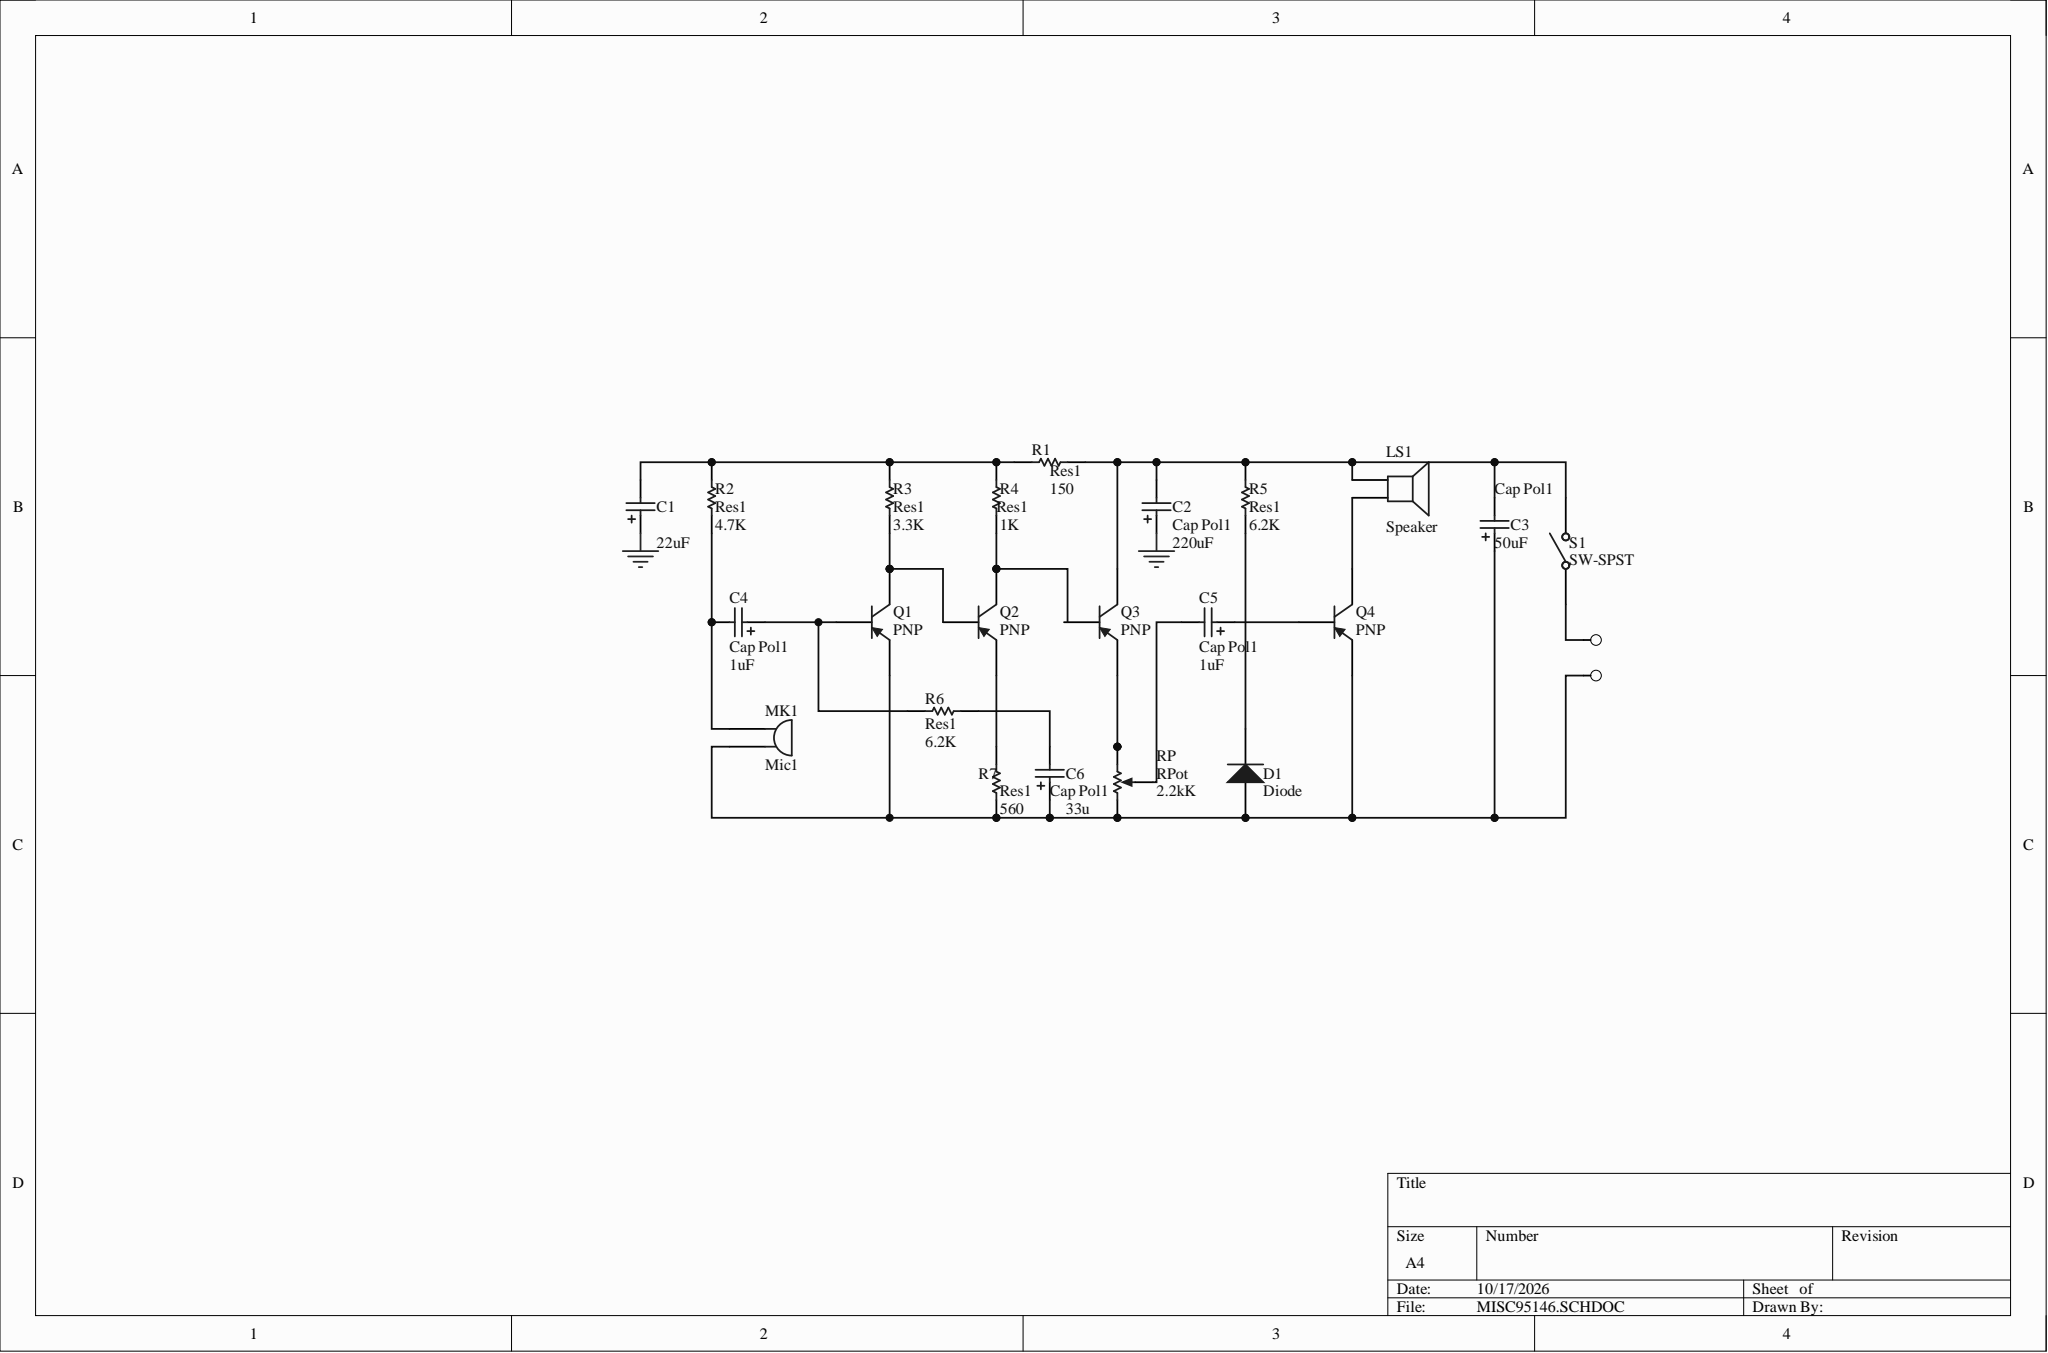Circuit board | Altium Designer | 22 parts | 15 nets
Bill of materials:
Comment,Description,Designator,Footprint,LibRef,Quantity
"Cap Pol1","Polarized Capacitor (Radial)","C1, C2, C3, C4, C5, C6","RB7.6-15","Cap Pol1","6"
"Diode","Default Diode","D1","DSO-C2/X3.3","Diode","1"
"Speaker","Loudspeaker","LS1","PIN2","Speaker","1"
"Mic1","Microphone","MK1","PIN2","Mic1","1"
"PNP","PNP Bipolar Transistor","Q1, Q2, Q3, Q4","SO-G3/C2.5","PNP","4"
"Res1","Resistor","R1, R2, R3, R4, R5, R6, R7","AXIAL-0.3","Res1","7"
"RPot","Potentiometer","RP","VR2","RPot","1"
"SW-SPST","Single-Pole, Single-Throw Switch","S1","SPST-2","SW-SPST","1"
Netlist (Protel format):
[
C1
RB7.6-15
Cap Pol1



]
[
C2
RB7.6-15
Cap Pol1



]
[
C3
RB7.6-15
Cap Pol1



]
[
C4
RB7.6-15
Cap Pol1



]
[
C5
RB7.6-15
Cap Pol1



]
[
C6
RB7.6-15
Cap Pol1



]
[
D1
DSO-C2/X3.3
Diode



]
[
LS1
PIN2
Speaker



]
[
MK1
PIN2
Mic1



]
[
Q1
SO-G3/C2.5
PNP



]
[
Q2
SO-G3/C2.5
PNP



]
[
Q3
SO-G3/C2.5
PNP



]
[
Q4
SO-G3/C2.5
PNP



]
[
R1
AXIAL-0.3
Res1



]
[
R2
AXIAL-0.3
Res1



]
[
R3
AXIAL-0.3
Res1



]
[
R4
AXIAL-0.3
Res1



]
[
R5
AXIAL-0.3
Res1



]
[
R6
AXIAL-0.3
Res1



]
[
R7
AXIAL-0.3
Res1



]
[
RP
VR2
RPot



]
[
S1
SPST-2
SW-SPST



]
(
NetQ3_3
Q3-3
RP-2
)
(
NetQ2_3
Q2-3
R7-2
)
(
NetQ2_1
Q2-1
R4-1
)
(
NetQ1_1
Q1-1
Q2-2
R3-1
)
(
NetLS1_2
LS1-2
Q4-1
)
(
NetD1_2
D1-2
R5-1
)
(
NetC6_2
C6-2
R6-1
)
(
NetC5_2
C5-2
RP-3
)
(
NetC5_1
C5-1
Q4-2
)
(
NetC4_2
C4-2
MK1-1
R2-1
)
(
NetC4_1
C4-1
Q1-2
R6-2
)
(
NetC3_1
C3-1
C6-1
D1-1
MK1-2
Q1-3
Q4-3
R7-1
RP-1
S1-1
)
(
NetC2_2
C2-2
C3-2
LS1-1
Q3-1
R1-2
R5-2
S1-2
)
(
NetC1_2
C1-2
R1-1
R2-2
R3-2
R4-2
)
(
GND
C1-1
C2-1
)